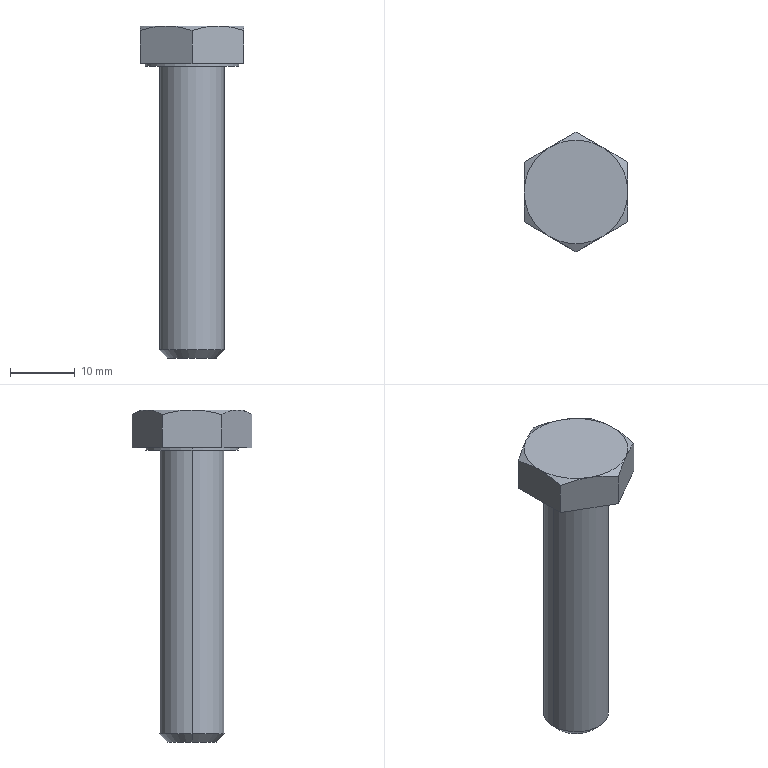Part | SolidWorks | features ICE 3, Chamfer 1, Extrusion 1, Fillet 1, RefAxis 1 | 1 solid | 24 faces | box 16 x 18.475 x 51.2 mm | volume 4858 mm3 | plane 10 | cone 8 | cylinder 4 | torus 2 | commonest cylinder face diameters 10 x2 14.4 x2
STEP:
#1=CARTESIAN_POINT('',(-5.1,0.,0.));
#2=VERTEX_POINT('',#1);
#3=CARTESIAN_POINT('',(5.1,0.,0.));
#4=VERTEX_POINT('',#3);
#5=CARTESIAN_POINT('',(0.,0.,0.));
#6=DIRECTION('',(0.,0.,1.));
#7=DIRECTION('',(1.,0.,0.));
#8=AXIS2_PLACEMENT_3D('',#5,#6,#7);
#9=CIRCLE('',#8,5.1);
#10=EDGE_CURVE('',#2,#4,#9,.T.);
#11=ORIENTED_EDGE('',*,*,#10,.F.);
#12=CARTESIAN_POINT('',(-5.,0.,-0.1));
#13=VERTEX_POINT('',#12);
#14=CARTESIAN_POINT('',(-5.1,0.,-0.1));
#15=DIRECTION('',(0.,1.,0.));
#16=DIRECTION('',(-1.,0.,0.));
#17=AXIS2_PLACEMENT_3D('',#14,#15,#16);
#18=CIRCLE('',#17,0.1);
#19=EDGE_CURVE('',#2,#13,#18,.T.);
#20=ORIENTED_EDGE('',*,*,#19,.T.);
#21=CARTESIAN_POINT('',(5.,0.,-0.1));
#22=VERTEX_POINT('',#21);
#23=CARTESIAN_POINT('',(0.,0.,-0.1));
#24=DIRECTION('',(0.,0.,-1.));
#25=DIRECTION('',(1.,0.,0.));
#26=AXIS2_PLACEMENT_3D('',#23,#24,#25);
#27=CIRCLE('',#26,5.);
#28=EDGE_CURVE('',#22,#13,#27,.T.);
#29=ORIENTED_EDGE('',*,*,#28,.F.);
#30=CARTESIAN_POINT('',(5.1,0.,-0.1));
#31=DIRECTION('',(0.,-1.,0.));
#32=DIRECTION('',(0.,0.,-1.));
#33=AXIS2_PLACEMENT_3D('',#30,#31,#32);
#34=CIRCLE('',#33,0.1);
#35=EDGE_CURVE('',#4,#22,#34,.T.);
#36=ORIENTED_EDGE('',*,*,#35,.F.);
#37=EDGE_LOOP('',(#11,#20,#29,#36));
#38=FACE_OUTER_BOUND('',#37,.T.);
#39=CARTESIAN_POINT('',(0.,0.,-0.1));
#40=DIRECTION('',(0.,0.,1.));
#41=DIRECTION('',(1.,0.,0.));
#42=AXIS2_PLACEMENT_3D('',#39,#40,#41);
#43=TOROIDAL_SURFACE('',#42,5.1,0.1);
#44=ADVANCED_FACE('',(#38),#43,.F.);
#45=CARTESIAN_POINT('',(7.2,0.,0.4133));
#46=VERTEX_POINT('',#45);
#47=CARTESIAN_POINT('',(-7.2,0.,0.4133));
#48=VERTEX_POINT('',#47);
#49=CARTESIAN_POINT('',(0.,0.,0.4133));
#50=DIRECTION('',(0.,0.,1.));
#51=DIRECTION('',(1.,0.,0.));
#52=AXIS2_PLACEMENT_3D('',#49,#50,#51);
#53=CIRCLE('',#52,7.2);
#54=EDGE_CURVE('',#46,#48,#53,.T.);
#55=ORIENTED_EDGE('',*,*,#54,.F.);
#56=CARTESIAN_POINT('',(7.2,0.,0.));
#57=VERTEX_POINT('',#56);
#58=CARTESIAN_POINT('',(7.2,0.,0.4133));
#59=DIRECTION('',(0.,0.,-1.));
#60=VECTOR('',#59,1000.);
#61=LINE('',#58,#60);
#62=EDGE_CURVE('',#46,#57,#61,.T.);
#63=ORIENTED_EDGE('',*,*,#62,.T.);
#64=CARTESIAN_POINT('',(-7.2,0.,0.));
#65=VERTEX_POINT('',#64);
#66=CARTESIAN_POINT('',(0.,0.,0.));
#67=DIRECTION('',(0.,0.,1.));
#68=DIRECTION('',(1.,0.,0.));
#69=AXIS2_PLACEMENT_3D('',#66,#67,#68);
#70=CIRCLE('',#69,7.2);
#71=EDGE_CURVE('',#57,#65,#70,.T.);
#72=ORIENTED_EDGE('',*,*,#71,.T.);
#73=CARTESIAN_POINT('',(-7.2,0.,0.4133));
#74=DIRECTION('',(0.,0.,-1.));
#75=VECTOR('',#74,1000.);
#76=LINE('',#73,#75);
#77=EDGE_CURVE('',#48,#65,#76,.T.);
#78=ORIENTED_EDGE('',*,*,#77,.F.);
#79=EDGE_LOOP('',(#55,#63,#72,#78));
#80=FACE_OUTER_BOUND('',#79,.T.);
#81=CARTESIAN_POINT('',(0.,0.,0.4133));
#82=DIRECTION('',(0.,0.,-1.));
#83=DIRECTION('',(-1.,0.,0.));
#84=AXIS2_PLACEMENT_3D('',#81,#82,#83);
#85=CYLINDRICAL_SURFACE('',#84,7.2);
#86=ADVANCED_FACE('',(#80),#85,.T.);
#87=CARTESIAN_POINT('',(-3.75,0.,-45.));
#88=VERTEX_POINT('',#87);
#89=CARTESIAN_POINT('',(3.75,0.,-45.));
#90=VERTEX_POINT('',#89);
#91=CARTESIAN_POINT('',(0.,0.,-45.));
#92=DIRECTION('',(0.,0.,-1.));
#93=DIRECTION('',(1.,0.,0.));
#94=AXIS2_PLACEMENT_3D('',#91,#92,#93);
#95=CIRCLE('',#94,3.75);
#96=EDGE_CURVE('',#88,#90,#95,.T.);
#97=ORIENTED_EDGE('',*,*,#96,.F.);
#98=CARTESIAN_POINT('',(-5.,0.,-43.75));
#99=VERTEX_POINT('',#98);
#100=CARTESIAN_POINT('',(-5.,0.,-43.75));
#101=DIRECTION('',(-0.7071,0.,0.7071));
#102=VECTOR('',#101,1000.);
#103=LINE('',#100,#102);
#104=EDGE_CURVE('',#88,#99,#103,.T.);
#105=ORIENTED_EDGE('',*,*,#104,.T.);
#106=CARTESIAN_POINT('',(5.,0.,-43.75));
#107=VERTEX_POINT('',#106);
#108=CARTESIAN_POINT('',(0.,0.,-43.75));
#109=DIRECTION('',(0.,0.,1.));
#110=DIRECTION('',(1.,0.,0.));
#111=AXIS2_PLACEMENT_3D('',#108,#109,#110);
#112=CIRCLE('',#111,5.);
#113=EDGE_CURVE('',#107,#99,#112,.T.);
#114=ORIENTED_EDGE('',*,*,#113,.F.);
#115=CARTESIAN_POINT('',(5.,0.,-43.75));
#116=DIRECTION('',(0.7071,0.,0.7071));
#117=VECTOR('',#116,1000.);
#118=LINE('',#115,#117);
#119=EDGE_CURVE('',#90,#107,#118,.T.);
#120=ORIENTED_EDGE('',*,*,#119,.F.);
#121=EDGE_LOOP('',(#97,#105,#114,#120));
#122=FACE_OUTER_BOUND('',#121,.T.);
#123=CARTESIAN_POINT('',(0.,0.,-43.75));
#124=DIRECTION('',(0.,0.,1.));
#125=DIRECTION('',(1.,0.,0.));
#126=AXIS2_PLACEMENT_3D('',#123,#124,#125);
#127=CONICAL_SURFACE('',#126,5.,0.7854);
#128=ADVANCED_FACE('',(#122),#127,.T.);
#129=ORIENTED_EDGE('',*,*,#113,.T.);
#130=CARTESIAN_POINT('',(-5.,0.,-45.));
#131=DIRECTION('',(0.,0.,1.));
#132=VECTOR('',#131,1000.);
#133=LINE('',#130,#132);
#134=EDGE_CURVE('',#99,#13,#133,.T.);
#135=ORIENTED_EDGE('',*,*,#134,.T.);
#136=CARTESIAN_POINT('',(0.,0.,-0.1));
#137=DIRECTION('',(0.,0.,-1.));
#138=DIRECTION('',(1.,0.,0.));
#139=AXIS2_PLACEMENT_3D('',#136,#137,#138);
#140=CIRCLE('',#139,5.);
#141=EDGE_CURVE('',#13,#22,#140,.T.);
#142=ORIENTED_EDGE('',*,*,#141,.T.);
#143=CARTESIAN_POINT('',(5.,0.,-45.));
#144=DIRECTION('',(0.,0.,1.));
#145=VECTOR('',#144,1000.);
#146=LINE('',#143,#145);
#147=EDGE_CURVE('',#107,#22,#146,.T.);
#148=ORIENTED_EDGE('',*,*,#147,.F.);
#149=EDGE_LOOP('',(#129,#135,#142,#148));
#150=FACE_OUTER_BOUND('',#149,.T.);
#151=CARTESIAN_POINT('',(0.,0.,-45.));
#152=DIRECTION('',(0.,0.,1.));
#153=DIRECTION('',(1.,0.,0.));
#154=AXIS2_PLACEMENT_3D('',#151,#152,#153);
#155=CYLINDRICAL_SURFACE('',#154,5.);
#156=ADVANCED_FACE('',(#150),#155,.T.);
#157=CARTESIAN_POINT('',(0.,0.,0.));
#158=DIRECTION('',(0.,0.,1.));
#159=DIRECTION('',(1.,0.,0.));
#160=AXIS2_PLACEMENT_3D('',#157,#158,#159);
#161=CIRCLE('',#160,5.1);
#162=EDGE_CURVE('',#4,#2,#161,.T.);
#163=ORIENTED_EDGE('',*,*,#162,.T.);
#164=ORIENTED_EDGE('',*,*,#10,.T.);
#165=EDGE_LOOP('',(#163,#164));
#166=FACE_BOUND('',#165,.T.);
#167=CARTESIAN_POINT('',(0.,0.,0.));
#168=DIRECTION('',(0.,0.,1.));
#169=DIRECTION('',(1.,0.,0.));
#170=AXIS2_PLACEMENT_3D('',#167,#168,#169);
#171=CIRCLE('',#170,7.2);
#172=EDGE_CURVE('',#65,#57,#171,.T.);
#173=ORIENTED_EDGE('',*,*,#172,.F.);
#174=ORIENTED_EDGE('',*,*,#71,.F.);
#175=EDGE_LOOP('',(#173,#174));
#176=FACE_OUTER_BOUND('',#175,.T.);
#177=CARTESIAN_POINT('',(0.,0.,0.));
#178=DIRECTION('',(0.,0.,1.));
#179=DIRECTION('',(1.,0.,0.));
#180=AXIS2_PLACEMENT_3D('',#177,#178,#179);
#181=PLANE('',#180);
#182=ADVANCED_FACE('',(#166,#176),#181,.F.);
#183=ORIENTED_EDGE('',*,*,#134,.F.);
#184=CARTESIAN_POINT('',(0.,0.,-43.75));
#185=DIRECTION('',(0.,0.,1.));
#186=DIRECTION('',(1.,0.,0.));
#187=AXIS2_PLACEMENT_3D('',#184,#185,#186);
#188=CIRCLE('',#187,5.);
#189=EDGE_CURVE('',#99,#107,#188,.T.);
#190=ORIENTED_EDGE('',*,*,#189,.T.);
#191=ORIENTED_EDGE('',*,*,#147,.T.);
#192=ORIENTED_EDGE('',*,*,#28,.T.);
#193=EDGE_LOOP('',(#183,#190,#191,#192));
#194=FACE_OUTER_BOUND('',#193,.T.);
#195=CARTESIAN_POINT('',(0.,0.,-45.));
#196=DIRECTION('',(0.,0.,1.));
#197=DIRECTION('',(1.,0.,0.));
#198=AXIS2_PLACEMENT_3D('',#195,#196,#197);
#199=CYLINDRICAL_SURFACE('',#198,5.);
#200=ADVANCED_FACE('',(#194),#199,.T.);
#201=CARTESIAN_POINT('',(0.,0.,-45.));
#202=DIRECTION('',(0.,0.,-1.));
#203=DIRECTION('',(1.,0.,0.));
#204=AXIS2_PLACEMENT_3D('',#201,#202,#203);
#205=CIRCLE('',#204,3.75);
#206=EDGE_CURVE('',#90,#88,#205,.T.);
#207=ORIENTED_EDGE('',*,*,#206,.T.);
#208=ORIENTED_EDGE('',*,*,#96,.T.);
#209=EDGE_LOOP('',(#207,#208));
#210=FACE_OUTER_BOUND('',#209,.T.);
#211=CARTESIAN_POINT('',(0.,0.,-45.));
#212=DIRECTION('',(0.,0.,1.));
#213=DIRECTION('',(1.,0.,0.));
#214=AXIS2_PLACEMENT_3D('',#211,#212,#213);
#215=PLANE('',#214);
#216=ADVANCED_FACE('',(#210),#215,.F.);
#217=ORIENTED_EDGE('',*,*,#104,.F.);
#218=ORIENTED_EDGE('',*,*,#206,.F.);
#219=ORIENTED_EDGE('',*,*,#119,.T.);
#220=ORIENTED_EDGE('',*,*,#189,.F.);
#221=EDGE_LOOP('',(#217,#218,#219,#220));
#222=FACE_OUTER_BOUND('',#221,.T.);
#223=CARTESIAN_POINT('',(0.,0.,-43.75));
#224=DIRECTION('',(0.,0.,1.));
#225=DIRECTION('',(1.,0.,0.));
#226=AXIS2_PLACEMENT_3D('',#223,#224,#225);
#227=CONICAL_SURFACE('',#226,5.,0.7854);
#228=ADVANCED_FACE('',(#222),#227,.T.);
#229=CARTESIAN_POINT('',(0.,0.,0.4133));
#230=DIRECTION('',(0.,0.,1.));
#231=DIRECTION('',(1.,0.,0.));
#232=AXIS2_PLACEMENT_3D('',#229,#230,#231);
#233=CIRCLE('',#232,7.2);
#234=EDGE_CURVE('',#48,#46,#233,.T.);
#235=ORIENTED_EDGE('',*,*,#234,.T.);
#236=ORIENTED_EDGE('',*,*,#54,.T.);
#237=EDGE_LOOP('',(#235,#236));
#238=FACE_BOUND('',#237,.T.);
#239=CARTESIAN_POINT('',(8.,-4.619,0.4133));
#240=VERTEX_POINT('',#239);
#241=CARTESIAN_POINT('',(8.,4.619,0.4133));
#242=VERTEX_POINT('',#241);
#243=CARTESIAN_POINT('',(8.,-4.619,0.4133));
#244=DIRECTION('',(0.,1.,0.));
#245=VECTOR('',#244,1000.);
#246=LINE('',#243,#245);
#247=EDGE_CURVE('',#240,#242,#246,.T.);
#248=ORIENTED_EDGE('',*,*,#247,.F.);
#249=CARTESIAN_POINT('',(0.,-9.238,0.4133));
#250=VERTEX_POINT('',#249);
#251=CARTESIAN_POINT('',(0.,-9.238,0.4133));
#252=DIRECTION('',(0.866,0.5,0.));
#253=VECTOR('',#252,1000.);
#254=LINE('',#251,#253);
#255=EDGE_CURVE('',#250,#240,#254,.T.);
#256=ORIENTED_EDGE('',*,*,#255,.F.);
#257=CARTESIAN_POINT('',(-8.,-4.619,0.4133));
#258=VERTEX_POINT('',#257);
#259=CARTESIAN_POINT('',(-8.,-4.619,0.4133));
#260=DIRECTION('',(0.866,-0.5,0.));
#261=VECTOR('',#260,1000.);
#262=LINE('',#259,#261);
#263=EDGE_CURVE('',#258,#250,#262,.T.);
#264=ORIENTED_EDGE('',*,*,#263,.F.);
#265=CARTESIAN_POINT('',(-8.,4.619,0.4133));
#266=VERTEX_POINT('',#265);
#267=CARTESIAN_POINT('',(-8.,4.619,0.4133));
#268=DIRECTION('',(0.,-1.,0.));
#269=VECTOR('',#268,1000.);
#270=LINE('',#267,#269);
#271=EDGE_CURVE('',#266,#258,#270,.T.);
#272=ORIENTED_EDGE('',*,*,#271,.F.);
#273=CARTESIAN_POINT('',(0.,9.238,0.4133));
#274=VERTEX_POINT('',#273);
#275=CARTESIAN_POINT('',(0.,9.238,0.4133));
#276=DIRECTION('',(-0.866,-0.5,0.));
#277=VECTOR('',#276,1000.);
#278=LINE('',#275,#277);
#279=EDGE_CURVE('',#274,#266,#278,.T.);
#280=ORIENTED_EDGE('',*,*,#279,.F.);
#281=CARTESIAN_POINT('',(8.,4.619,0.4133));
#282=DIRECTION('',(-0.866,0.5,0.));
#283=VECTOR('',#282,1000.);
#284=LINE('',#281,#283);
#285=EDGE_CURVE('',#242,#274,#284,.T.);
#286=ORIENTED_EDGE('',*,*,#285,.F.);
#287=EDGE_LOOP('',(#248,#256,#264,#272,#280,#286));
#288=FACE_OUTER_BOUND('',#287,.T.);
#289=CARTESIAN_POINT('',(0.,0.,0.4133));
#290=DIRECTION('',(0.,0.,1.));
#291=DIRECTION('',(1.,0.,0.));
#292=AXIS2_PLACEMENT_3D('',#289,#290,#291);
#293=PLANE('',#292);
#294=ADVANCED_FACE('',(#238,#288),#293,.F.);
#295=ORIENTED_EDGE('',*,*,#62,.F.);
#296=ORIENTED_EDGE('',*,*,#234,.F.);
#297=ORIENTED_EDGE('',*,*,#77,.T.);
#298=ORIENTED_EDGE('',*,*,#172,.T.);
#299=EDGE_LOOP('',(#295,#296,#297,#298));
#300=FACE_OUTER_BOUND('',#299,.T.);
#301=CARTESIAN_POINT('',(0.,0.,0.4133));
#302=DIRECTION('',(0.,0.,-1.));
#303=DIRECTION('',(-1.,0.,0.));
#304=AXIS2_PLACEMENT_3D('',#301,#302,#303);
#305=CYLINDRICAL_SURFACE('',#304,7.2);
#306=ADVANCED_FACE('',(#300),#305,.T.);
#307=CARTESIAN_POINT('',(4.,-6.928,6.2));
#308=VERTEX_POINT('',#307);
#309=CARTESIAN_POINT('',(8.,0.,6.2));
#310=VERTEX_POINT('',#309);
#311=CARTESIAN_POINT('',(0.,0.,6.2));
#312=DIRECTION('',(0.,0.,1.));
#313=DIRECTION('',(1.,0.,0.));
#314=AXIS2_PLACEMENT_3D('',#311,#312,#313);
#315=CIRCLE('',#314,8.);
#316=EDGE_CURVE('',#308,#310,#315,.T.);
#317=ORIENTED_EDGE('',*,*,#316,.T.);
#318=CARTESIAN_POINT('',(4.,6.928,6.2));
#319=VERTEX_POINT('',#318);
#320=CARTESIAN_POINT('',(0.,0.,6.2));
#321=DIRECTION('',(0.,0.,1.));
#322=DIRECTION('',(1.,0.,0.));
#323=AXIS2_PLACEMENT_3D('',#320,#321,#322);
#324=CIRCLE('',#323,8.);
#325=EDGE_CURVE('',#310,#319,#324,.T.);
#326=ORIENTED_EDGE('',*,*,#325,.T.);
#327=CARTESIAN_POINT('',(-4.,6.928,6.2));
#328=VERTEX_POINT('',#327);
#329=CARTESIAN_POINT('',(0.,0.,6.2));
#330=DIRECTION('',(0.,0.,1.));
#331=DIRECTION('',(1.,0.,0.));
#332=AXIS2_PLACEMENT_3D('',#329,#330,#331);
#333=CIRCLE('',#332,8.);
#334=EDGE_CURVE('',#319,#328,#333,.T.);
#335=ORIENTED_EDGE('',*,*,#334,.T.);
#336=CARTESIAN_POINT('',(-8.,0.,6.2));
#337=VERTEX_POINT('',#336);
#338=CARTESIAN_POINT('',(0.,0.,6.2));
#339=DIRECTION('',(0.,0.,1.));
#340=DIRECTION('',(1.,0.,0.));
#341=AXIS2_PLACEMENT_3D('',#338,#339,#340);
#342=CIRCLE('',#341,8.);
#343=EDGE_CURVE('',#328,#337,#342,.T.);
#344=ORIENTED_EDGE('',*,*,#343,.T.);
#345=CARTESIAN_POINT('',(-4.,-6.928,6.2));
#346=VERTEX_POINT('',#345);
#347=CARTESIAN_POINT('',(0.,0.,6.2));
#348=DIRECTION('',(0.,0.,1.));
#349=DIRECTION('',(1.,0.,0.));
#350=AXIS2_PLACEMENT_3D('',#347,#348,#349);
#351=CIRCLE('',#350,8.);
#352=EDGE_CURVE('',#337,#346,#351,.T.);
#353=ORIENTED_EDGE('',*,*,#352,.T.);
#354=CARTESIAN_POINT('',(0.,0.,6.2));
#355=DIRECTION('',(0.,0.,1.));
#356=DIRECTION('',(1.,0.,0.));
#357=AXIS2_PLACEMENT_3D('',#354,#355,#356);
#358=CIRCLE('',#357,8.);
#359=EDGE_CURVE('',#346,#308,#358,.T.);
#360=ORIENTED_EDGE('',*,*,#359,.T.);
#361=EDGE_LOOP('',(#317,#326,#335,#344,#353,#360));
#362=FACE_OUTER_BOUND('',#361,.T.);
#363=CARTESIAN_POINT('',(0.,0.,6.2));
#364=DIRECTION('',(0.,0.,1.));
#365=DIRECTION('',(1.,0.,0.));
#366=AXIS2_PLACEMENT_3D('',#363,#364,#365);
#367=PLANE('',#366);
#368=ADVANCED_FACE('',(#362),#367,.T.);
#369=CARTESIAN_POINT('',(0.,9.238,5.485));
#370=VERTEX_POINT('',#369);
#371=CARTESIAN_POINT('',(4.,6.928,6.2));
#372=CARTESIAN_POINT('',(3.661,7.124,6.2));
#373=CARTESIAN_POINT('',(3.32,7.321,6.183));
#374=CARTESIAN_POINT('',(2.645,7.711,6.118));
#375=CARTESIAN_POINT('',(2.31,7.904,6.069));
#376=CARTESIAN_POINT('',(1.311,8.481,5.883));
#377=CARTESIAN_POINT('',(0.6527,8.861,5.703));
#378=CARTESIAN_POINT('',(0.,9.238,5.485));
#379=B_SPLINE_CURVE_WITH_KNOTS('',3,(#371,#372,#373,#374,#375,#376,#377,#378),.UNSPECIFIED.,.F.,.F.,(4,2,2,4),(0.004674,0.005838,0.007002,0.00933),.UNSPECIFIED.);
#380=EDGE_CURVE('',#319,#370,#379,.T.);
#381=ORIENTED_EDGE('',*,*,#380,.T.);
#382=CARTESIAN_POINT('',(0.,9.238,5.485));
#383=CARTESIAN_POINT('',(-0.6543,8.86,5.704));
#384=CARTESIAN_POINT('',(-1.313,8.479,5.883));
#385=CARTESIAN_POINT('',(-2.646,7.71,6.132));
#386=CARTESIAN_POINT('',(-3.319,7.322,6.2));
#387=CARTESIAN_POINT('',(-4.,6.928,6.2));
#388=B_SPLINE_CURVE_WITH_KNOTS('',3,(#382,#383,#384,#385,#386,#387),.UNSPECIFIED.,.F.,.F.,(4,2,4),(0.000000238,0.002337,0.004674),.UNSPECIFIED.);
#389=EDGE_CURVE('',#370,#328,#388,.T.);
#390=ORIENTED_EDGE('',*,*,#389,.T.);
#391=ORIENTED_EDGE('',*,*,#334,.F.);
#392=EDGE_LOOP('',(#381,#390,#391));
#393=FACE_OUTER_BOUND('',#392,.T.);
#394=CARTESIAN_POINT('',(0.,0.,6.2));
#395=DIRECTION('',(0.,0.,-1.));
#396=DIRECTION('',(1.,0.,0.));
#397=AXIS2_PLACEMENT_3D('',#394,#395,#396);
#398=CONICAL_SURFACE('',#397,8.,1.047);
#399=ADVANCED_FACE('',(#393),#398,.T.);
#400=CARTESIAN_POINT('',(-8.,4.619,5.485));
#401=VERTEX_POINT('',#400);
#402=CARTESIAN_POINT('',(-4.,6.928,6.2));
#403=CARTESIAN_POINT('',(-4.339,6.732,6.2));
#404=CARTESIAN_POINT('',(-4.68,6.535,6.183));
#405=CARTESIAN_POINT('',(-5.355,6.146,6.118));
#406=CARTESIAN_POINT('',(-5.69,5.952,6.069));
#407=CARTESIAN_POINT('',(-6.689,5.376,5.883));
#408=CARTESIAN_POINT('',(-7.347,4.996,5.703));
#409=CARTESIAN_POINT('',(-8.,4.619,5.485));
#410=B_SPLINE_CURVE_WITH_KNOTS('',3,(#402,#403,#404,#405,#406,#407,#408,#409),.UNSPECIFIED.,.F.,.F.,(4,2,2,4),(0.004674,0.005838,0.007002,0.00933),.UNSPECIFIED.);
#411=EDGE_CURVE('',#328,#401,#410,.T.);
#412=ORIENTED_EDGE('',*,*,#411,.T.);
#413=CARTESIAN_POINT('',(-8.,4.619,5.485));
#414=CARTESIAN_POINT('',(-8.,3.872,5.701));
#415=CARTESIAN_POINT('',(-8.,3.115,5.881));
#416=CARTESIAN_POINT('',(-8.,1.959,6.068));
#417=CARTESIAN_POINT('',(-8.,1.571,6.117));
#418=CARTESIAN_POINT('',(-8.,0.7848,6.183));
#419=CARTESIAN_POINT('',(-8.,0.3911,6.2));
#420=CARTESIAN_POINT('',(-8.,0.,6.2));
#421=B_SPLINE_CURVE_WITH_KNOTS('',3,(#413,#414,#415,#416,#417,#418,#419,#420),.UNSPECIFIED.,.F.,.F.,(4,2,2,4),(0.02459,0.02692,0.02809,0.02926),.UNSPECIFIED.);
#422=EDGE_CURVE('',#401,#337,#421,.T.);
#423=ORIENTED_EDGE('',*,*,#422,.T.);
#424=ORIENTED_EDGE('',*,*,#343,.F.);
#425=EDGE_LOOP('',(#412,#423,#424));
#426=FACE_OUTER_BOUND('',#425,.T.);
#427=CARTESIAN_POINT('',(0.,0.,6.2));
#428=DIRECTION('',(0.,0.,-1.));
#429=DIRECTION('',(1.,0.,0.));
#430=AXIS2_PLACEMENT_3D('',#427,#428,#429);
#431=CONICAL_SURFACE('',#430,8.,1.047);
#432=ADVANCED_FACE('',(#426),#431,.T.);
#433=CARTESIAN_POINT('',(-8.,-4.619,5.485));
#434=VERTEX_POINT('',#433);
#435=CARTESIAN_POINT('',(-8.,0.,6.2));
#436=CARTESIAN_POINT('',(-8.,-0.7816,6.2));
#437=CARTESIAN_POINT('',(-8.,-1.557,6.133));
#438=CARTESIAN_POINT('',(-8.,-3.098,5.884));
#439=CARTESIAN_POINT('',(-8.,-3.867,5.703));
#440=CARTESIAN_POINT('',(-8.,-4.619,5.485));
#441=B_SPLINE_CURVE_WITH_KNOTS('',3,(#435,#436,#437,#438,#439,#440),.UNSPECIFIED.,.F.,.F.,(4,2,4),(0.02926,0.0316,0.03394),.UNSPECIFIED.);
#442=EDGE_CURVE('',#337,#434,#441,.T.);
#443=ORIENTED_EDGE('',*,*,#442,.T.);
#444=CARTESIAN_POINT('',(-8.,-4.619,5.485));
#445=CARTESIAN_POINT('',(-7.346,-4.997,5.704));
#446=CARTESIAN_POINT('',(-6.687,-5.377,5.883));
#447=CARTESIAN_POINT('',(-5.354,-6.146,6.132));
#448=CARTESIAN_POINT('',(-4.681,-6.535,6.2));
#449=CARTESIAN_POINT('',(-4.,-6.928,6.2));
#450=B_SPLINE_CURVE_WITH_KNOTS('',3,(#444,#445,#446,#447,#448,#449),.UNSPECIFIED.,.F.,.F.,(4,2,4),(0.000000238,0.002337,0.004674),.UNSPECIFIED.);
#451=EDGE_CURVE('',#434,#346,#450,.T.);
#452=ORIENTED_EDGE('',*,*,#451,.T.);
#453=ORIENTED_EDGE('',*,*,#352,.F.);
#454=EDGE_LOOP('',(#443,#452,#453));
#455=FACE_OUTER_BOUND('',#454,.T.);
#456=CARTESIAN_POINT('',(0.,0.,6.2));
#457=DIRECTION('',(0.,0.,-1.));
#458=DIRECTION('',(1.,0.,0.));
#459=AXIS2_PLACEMENT_3D('',#456,#457,#458);
#460=CONICAL_SURFACE('',#459,8.,1.047);
#461=ADVANCED_FACE('',(#455),#460,.T.);
#462=CARTESIAN_POINT('',(0.,-9.238,5.485));
#463=VERTEX_POINT('',#462);
#464=CARTESIAN_POINT('',(-4.,-6.928,6.2));
#465=CARTESIAN_POINT('',(-3.661,-7.124,6.2));
#466=CARTESIAN_POINT('',(-3.32,-7.321,6.183));
#467=CARTESIAN_POINT('',(-2.645,-7.711,6.118));
#468=CARTESIAN_POINT('',(-2.31,-7.904,6.069));
#469=CARTESIAN_POINT('',(-1.311,-8.481,5.883));
#470=CARTESIAN_POINT('',(-0.6527,-8.861,5.703));
#471=CARTESIAN_POINT('',(0.,-9.238,5.485));
#472=B_SPLINE_CURVE_WITH_KNOTS('',3,(#464,#465,#466,#467,#468,#469,#470,#471),.UNSPECIFIED.,.F.,.F.,(4,2,2,4),(0.004674,0.005838,0.007002,0.00933),.UNSPECIFIED.);
#473=EDGE_CURVE('',#346,#463,#472,.T.);
#474=ORIENTED_EDGE('',*,*,#473,.T.);
#475=CARTESIAN_POINT('',(0.,-9.238,5.485));
#476=CARTESIAN_POINT('',(0.6543,-8.86,5.704));
#477=CARTESIAN_POINT('',(1.313,-8.479,5.883));
#478=CARTESIAN_POINT('',(2.646,-7.71,6.132));
#479=CARTESIAN_POINT('',(3.319,-7.322,6.2));
#480=CARTESIAN_POINT('',(4.,-6.928,6.2));
#481=B_SPLINE_CURVE_WITH_KNOTS('',3,(#475,#476,#477,#478,#479,#480),.UNSPECIFIED.,.F.,.F.,(4,2,4),(0.000000238,0.002337,0.004674),.UNSPECIFIED.);
#482=EDGE_CURVE('',#463,#308,#481,.T.);
#483=ORIENTED_EDGE('',*,*,#482,.T.);
#484=ORIENTED_EDGE('',*,*,#359,.F.);
#485=EDGE_LOOP('',(#474,#483,#484));
#486=FACE_OUTER_BOUND('',#485,.T.);
#487=CARTESIAN_POINT('',(0.,0.,6.2));
#488=DIRECTION('',(0.,0.,-1.));
#489=DIRECTION('',(1.,0.,0.));
#490=AXIS2_PLACEMENT_3D('',#487,#488,#489);
#491=CONICAL_SURFACE('',#490,8.,1.047);
#492=ADVANCED_FACE('',(#486),#491,.T.);
#493=CARTESIAN_POINT('',(8.,-4.619,5.485));
#494=VERTEX_POINT('',#493);
#495=CARTESIAN_POINT('',(4.,-6.928,6.2));
#496=CARTESIAN_POINT('',(4.339,-6.732,6.2));
#497=CARTESIAN_POINT('',(4.68,-6.535,6.183));
#498=CARTESIAN_POINT('',(5.355,-6.146,6.118));
#499=CARTESIAN_POINT('',(5.69,-5.952,6.069));
#500=CARTESIAN_POINT('',(6.689,-5.376,5.883));
#501=CARTESIAN_POINT('',(7.347,-4.996,5.703));
#502=CARTESIAN_POINT('',(8.,-4.619,5.485));
#503=B_SPLINE_CURVE_WITH_KNOTS('',3,(#495,#496,#497,#498,#499,#500,#501,#502),.UNSPECIFIED.,.F.,.F.,(4,2,2,4),(0.004674,0.005838,0.007002,0.00933),.UNSPECIFIED.);
#504=EDGE_CURVE('',#308,#494,#503,.T.);
#505=ORIENTED_EDGE('',*,*,#504,.T.);
#506=CARTESIAN_POINT('',(8.,-4.619,5.485));
#507=CARTESIAN_POINT('',(8.,-3.867,5.703));
#508=CARTESIAN_POINT('',(8.,-3.098,5.884));
#509=CARTESIAN_POINT('',(8.,-1.557,6.133));
#510=CARTESIAN_POINT('',(8.,-0.7816,6.2));
#511=CARTESIAN_POINT('',(8.,0.,6.2));
#512=B_SPLINE_CURVE_WITH_KNOTS('',3,(#506,#507,#508,#509,#510,#511),.UNSPECIFIED.,.F.,.F.,(4,2,4),(0.008612,0.01095,0.01329),.UNSPECIFIED.);
#513=EDGE_CURVE('',#494,#310,#512,.T.);
#514=ORIENTED_EDGE('',*,*,#513,.T.);
#515=ORIENTED_EDGE('',*,*,#316,.F.);
#516=EDGE_LOOP('',(#505,#514,#515));
#517=FACE_OUTER_BOUND('',#516,.T.);
#518=CARTESIAN_POINT('',(0.,0.,6.2));
#519=DIRECTION('',(0.,0.,-1.));
#520=DIRECTION('',(1.,0.,0.));
#521=AXIS2_PLACEMENT_3D('',#518,#519,#520);
#522=CONICAL_SURFACE('',#521,8.,1.047);
#523=ADVANCED_FACE('',(#517),#522,.T.);
#524=CARTESIAN_POINT('',(8.,4.619,5.485));
#525=VERTEX_POINT('',#524);
#526=CARTESIAN_POINT('',(8.,4.619,5.485));
#527=CARTESIAN_POINT('',(7.346,4.997,5.704));
#528=CARTESIAN_POINT('',(6.687,5.377,5.883));
#529=CARTESIAN_POINT('',(5.354,6.146,6.132));
#530=CARTESIAN_POINT('',(4.681,6.535,6.2));
#531=CARTESIAN_POINT('',(4.,6.928,6.2));
#532=B_SPLINE_CURVE_WITH_KNOTS('',3,(#526,#527,#528,#529,#530,#531),.UNSPECIFIED.,.F.,.F.,(4,2,4),(0.000000238,0.002337,0.004674),.UNSPECIFIED.);
#533=EDGE_CURVE('',#525,#319,#532,.T.);
#534=ORIENTED_EDGE('',*,*,#533,.T.);
#535=ORIENTED_EDGE('',*,*,#325,.F.);
#536=CARTESIAN_POINT('',(8.,0.,6.2));
#537=CARTESIAN_POINT('',(8.,0.3911,6.2));
#538=CARTESIAN_POINT('',(8.,0.7848,6.183));
#539=CARTESIAN_POINT('',(8.,1.571,6.117));
#540=CARTESIAN_POINT('',(8.,1.959,6.068));
#541=CARTESIAN_POINT('',(8.,3.115,5.881));
#542=CARTESIAN_POINT('',(8.,3.872,5.701));
#543=CARTESIAN_POINT('',(8.,4.619,5.485));
#544=B_SPLINE_CURVE_WITH_KNOTS('',3,(#536,#537,#538,#539,#540,#541,#542,#543),.UNSPECIFIED.,.F.,.F.,(4,2,2,4),(0.01329,0.01446,0.01563,0.01797),.UNSPECIFIED.);
#545=EDGE_CURVE('',#310,#525,#544,.T.);
#546=ORIENTED_EDGE('',*,*,#545,.T.);
#547=EDGE_LOOP('',(#534,#535,#546));
#548=FACE_OUTER_BOUND('',#547,.T.);
#549=CARTESIAN_POINT('',(0.,0.,6.2));
#550=DIRECTION('',(0.,0.,-1.));
#551=DIRECTION('',(1.,0.,0.));
#552=AXIS2_PLACEMENT_3D('',#549,#550,#551);
#553=CONICAL_SURFACE('',#552,8.,1.047);
#554=ADVANCED_FACE('',(#548),#553,.T.);
#555=CARTESIAN_POINT('',(8.,-4.619,6.2));
#556=DIRECTION('',(0.,0.,-1.));
#557=VECTOR('',#556,1000.);
#558=LINE('',#555,#557);
#559=EDGE_CURVE('',#494,#240,#558,.T.);
#560=ORIENTED_EDGE('',*,*,#559,.T.);
#561=ORIENTED_EDGE('',*,*,#247,.T.);
#562=CARTESIAN_POINT('',(8.,4.619,6.2));
#563=DIRECTION('',(0.,0.,-1.));
#564=VECTOR('',#563,1000.);
#565=LINE('',#562,#564);
#566=EDGE_CURVE('',#525,#242,#565,.T.);
#567=ORIENTED_EDGE('',*,*,#566,.F.);
#568=ORIENTED_EDGE('',*,*,#545,.F.);
#569=ORIENTED_EDGE('',*,*,#513,.F.);
#570=EDGE_LOOP('',(#560,#561,#567,#568,#569));
#571=FACE_OUTER_BOUND('',#570,.T.);
#572=CARTESIAN_POINT('',(8.,-4.619,6.2));
#573=DIRECTION('',(-1.,0.,0.));
#574=DIRECTION('',(0.,-1.,0.));
#575=AXIS2_PLACEMENT_3D('',#572,#573,#574);
#576=PLANE('',#575);
#577=ADVANCED_FACE('',(#571),#576,.F.);
#578=CARTESIAN_POINT('',(0.,-9.238,6.2));
#579=DIRECTION('',(0.,0.,-1.));
#580=VECTOR('',#579,1000.);
#581=LINE('',#578,#580);
#582=EDGE_CURVE('',#463,#250,#581,.T.);
#583=ORIENTED_EDGE('',*,*,#582,.T.);
#584=ORIENTED_EDGE('',*,*,#255,.T.);
#585=ORIENTED_EDGE('',*,*,#559,.F.);
#586=ORIENTED_EDGE('',*,*,#504,.F.);
#587=ORIENTED_EDGE('',*,*,#482,.F.);
#588=EDGE_LOOP('',(#583,#584,#585,#586,#587));
#589=FACE_OUTER_BOUND('',#588,.T.);
#590=CARTESIAN_POINT('',(0.,-9.238,6.2));
#591=DIRECTION('',(-0.5,0.866,0.));
#592=DIRECTION('',(-0.866,-0.5,0.));
#593=AXIS2_PLACEMENT_3D('',#590,#591,#592);
#594=PLANE('',#593);
#595=ADVANCED_FACE('',(#589),#594,.F.);
#596=CARTESIAN_POINT('',(-8.,-4.619,6.2));
#597=DIRECTION('',(0.,0.,-1.));
#598=VECTOR('',#597,1000.);
#599=LINE('',#596,#598);
#600=EDGE_CURVE('',#434,#258,#599,.T.);
#601=ORIENTED_EDGE('',*,*,#600,.T.);
#602=ORIENTED_EDGE('',*,*,#263,.T.);
#603=ORIENTED_EDGE('',*,*,#582,.F.);
#604=ORIENTED_EDGE('',*,*,#473,.F.);
#605=ORIENTED_EDGE('',*,*,#451,.F.);
#606=EDGE_LOOP('',(#601,#602,#603,#604,#605));
#607=FACE_OUTER_BOUND('',#606,.T.);
#608=CARTESIAN_POINT('',(-8.,-4.619,6.2));
#609=DIRECTION('',(0.5,0.866,0.));
#610=DIRECTION('',(-0.866,0.5,0.));
#611=AXIS2_PLACEMENT_3D('',#608,#609,#610);
#612=PLANE('',#611);
#613=ADVANCED_FACE('',(#607),#612,.F.);
#614=CARTESIAN_POINT('',(-8.,4.619,6.2));
#615=DIRECTION('',(0.,0.,-1.));
#616=VECTOR('',#615,1000.);
#617=LINE('',#614,#616);
#618=EDGE_CURVE('',#401,#266,#617,.T.);
#619=ORIENTED_EDGE('',*,*,#618,.T.);
#620=ORIENTED_EDGE('',*,*,#271,.T.);
#621=ORIENTED_EDGE('',*,*,#600,.F.);
#622=ORIENTED_EDGE('',*,*,#442,.F.);
#623=ORIENTED_EDGE('',*,*,#422,.F.);
#624=EDGE_LOOP('',(#619,#620,#621,#622,#623));
#625=FACE_OUTER_BOUND('',#624,.T.);
#626=CARTESIAN_POINT('',(-8.,4.619,6.2));
#627=DIRECTION('',(1.,0.,0.));
#628=DIRECTION('',(0.,0.,-1.));
#629=AXIS2_PLACEMENT_3D('',#626,#627,#628);
#630=PLANE('',#629);
#631=ADVANCED_FACE('',(#625),#630,.F.);
#632=CARTESIAN_POINT('',(0.,9.238,6.2));
#633=DIRECTION('',(0.,0.,-1.));
#634=VECTOR('',#633,1000.);
#635=LINE('',#632,#634);
#636=EDGE_CURVE('',#370,#274,#635,.T.);
#637=ORIENTED_EDGE('',*,*,#636,.T.);
#638=ORIENTED_EDGE('',*,*,#279,.T.);
#639=ORIENTED_EDGE('',*,*,#618,.F.);
#640=ORIENTED_EDGE('',*,*,#411,.F.);
#641=ORIENTED_EDGE('',*,*,#389,.F.);
#642=EDGE_LOOP('',(#637,#638,#639,#640,#641));
#643=FACE_OUTER_BOUND('',#642,.T.);
#644=CARTESIAN_POINT('',(0.,9.238,6.2));
#645=DIRECTION('',(0.5,-0.866,0.));
#646=DIRECTION('',(0.866,0.5,0.));
#647=AXIS2_PLACEMENT_3D('',#644,#645,#646);
#648=PLANE('',#647);
#649=ADVANCED_FACE('',(#643),#648,.F.);
#650=ORIENTED_EDGE('',*,*,#566,.T.);
#651=ORIENTED_EDGE('',*,*,#285,.T.);
#652=ORIENTED_EDGE('',*,*,#636,.F.);
#653=ORIENTED_EDGE('',*,*,#380,.F.);
#654=ORIENTED_EDGE('',*,*,#533,.F.);
#655=EDGE_LOOP('',(#650,#651,#652,#653,#654));
#656=FACE_OUTER_BOUND('',#655,.T.);
#657=CARTESIAN_POINT('',(8.,4.619,6.2));
#658=DIRECTION('',(-0.5,-0.866,0.));
#659=DIRECTION('',(0.866,-0.5,0.));
#660=AXIS2_PLACEMENT_3D('',#657,#658,#659);
#661=PLANE('',#660);
#662=ADVANCED_FACE('',(#656),#661,.F.);
#663=ORIENTED_EDGE('',*,*,#19,.F.);
#664=ORIENTED_EDGE('',*,*,#162,.F.);
#665=ORIENTED_EDGE('',*,*,#35,.T.);
#666=ORIENTED_EDGE('',*,*,#141,.F.);
#667=EDGE_LOOP('',(#663,#664,#665,#666));
#668=FACE_OUTER_BOUND('',#667,.T.);
#669=CARTESIAN_POINT('',(0.,0.,-0.1));
#670=DIRECTION('',(0.,0.,1.));
#671=DIRECTION('',(1.,0.,0.));
#672=AXIS2_PLACEMENT_3D('',#669,#670,#671);
#673=TOROIDAL_SURFACE('',#672,5.1,0.1);
#674=ADVANCED_FACE('',(#668),#673,.F.);
#675=CLOSED_SHELL('',(#44,#86,#128,#156,#182,#200,#216,#228,#294,#306,#368,#399,#432,#461,#492,#523,#554,#577,#595,#613,#631,#649,#662,#674));
#676=MANIFOLD_SOLID_BREP('',#675);
#677=CARTESIAN_POINT('',(0.,0.,0.));
#678=DIRECTION('',(0.,0.,1.));
#679=DIRECTION('',(1.,0.,0.));
#680=AXIS2_PLACEMENT_3D('',#677,#678,#679);
#681=(LENGTH_UNIT()NAMED_UNIT(*)SI_UNIT(.MILLI.,.METRE.));
#682=UNCERTAINTY_MEASURE_WITH_UNIT(LENGTH_MEASURE(0.00001),#681,'','');
#683=(NAMED_UNIT(*)PLANE_ANGLE_UNIT()SI_UNIT($,.RADIAN.));
#684=(NAMED_UNIT(*)SI_UNIT($,.STERADIAN.)SOLID_ANGLE_UNIT());
#685=(GEOMETRIC_REPRESENTATION_CONTEXT(3)GLOBAL_UNCERTAINTY_ASSIGNED_CONTEXT((#682))GLOBAL_UNIT_ASSIGNED_CONTEXT((#681,#683,#684))REPRESENTATION_CONTEXT('',''));
#686=ADVANCED_BREP_SHAPE_REPRESENTATION('',(#676,#680),#685);